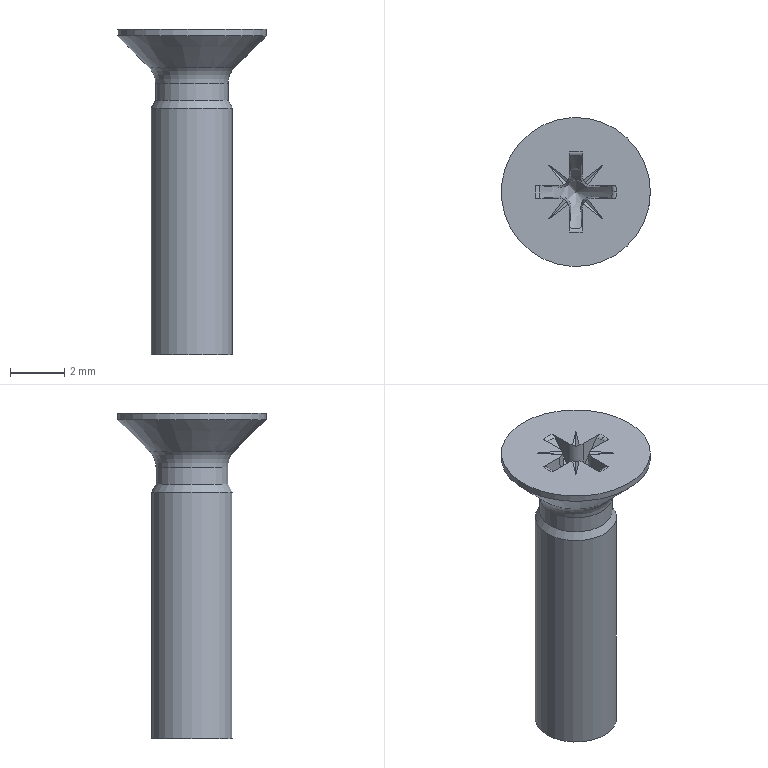Part | NX | features BREP 1, DATUM_CSYS 1 | 1 solid | 34 faces | box 5.5 x 5.5 x 12.001 mm | volume 94.702 mm3 | plane 18 | cylinder 7 | torus 6 | cone 3 | commonest cylinder face diameters 0.8 x4 2.675 x1 3 x1 5.5 x1
STEP:
#1=CARTESIAN_POINT('',(1.5,0.,-12.));
#2=VERTEX_POINT('',#1);
#3=CARTESIAN_POINT('',(0.,0.,-12.));
#4=DIRECTION('',(0.,0.,-1.));
#5=DIRECTION('',(1.,0.,0.));
#6=AXIS2_PLACEMENT_3D('',#3,#4,#5);
#7=CIRCLE('',#6,1.5);
#8=EDGE_CURVE('',#2,#2,#7,.T.);
#9=ORIENTED_EDGE('',*,*,#8,.T.);
#10=EDGE_LOOP('',(#9));
#11=FACE_BOUND('',#10,.T.);
#12=CARTESIAN_POINT('',(0.,0.,-12.));
#13=DIRECTION('',(0.,0.,-1.));
#14=DIRECTION('',(-1.,0.,0.));
#15=AXIS2_PLACEMENT_3D('',#12,#13,#14);
#16=PLANE('',#15);
#17=ADVANCED_FACE('',(#11),#16,.T.);
#18=CARTESIAN_POINT('',(1.5,0.,-2.9));
#19=VERTEX_POINT('',#18);
#20=CARTESIAN_POINT('',(1.5,0.,-12.));
#21=DIRECTION('',(0.,0.,1.));
#22=VECTOR('',#21,1000.);
#23=LINE('',#20,#22);
#24=EDGE_CURVE('',#2,#19,#23,.T.);
#25=ORIENTED_EDGE('',*,*,#24,.T.);
#26=CARTESIAN_POINT('',(0.,0.,-2.9));
#27=DIRECTION('',(0.,0.,-1.));
#28=DIRECTION('',(1.,0.,0.));
#29=AXIS2_PLACEMENT_3D('',#26,#27,#28);
#30=CIRCLE('',#29,1.5);
#31=EDGE_CURVE('',#19,#19,#30,.T.);
#32=ORIENTED_EDGE('',*,*,#31,.T.);
#33=ORIENTED_EDGE('',*,*,#24,.F.);
#34=ORIENTED_EDGE('',*,*,#8,.F.);
#35=EDGE_LOOP('',(#25,#32,#33,#34));
#36=FACE_BOUND('',#35,.T.);
#37=CARTESIAN_POINT('',(0.,0.,-12.));
#38=DIRECTION('',(0.,0.,1.));
#39=DIRECTION('',(-1.,0.,0.));
#40=AXIS2_PLACEMENT_3D('',#37,#38,#39);
#41=CYLINDRICAL_SURFACE('',#40,1.5);
#42=ADVANCED_FACE('',(#36),#41,.T.);
#43=CARTESIAN_POINT('',(1.338,0.,-2.619));
#44=VERTEX_POINT('',#43);
#45=CARTESIAN_POINT('',(1.5,0.,-2.9));
#46=DIRECTION('',(-0.5,0.,0.866));
#47=VECTOR('',#46,1000.);
#48=LINE('',#45,#47);
#49=EDGE_CURVE('',#19,#44,#48,.T.);
#50=ORIENTED_EDGE('',*,*,#49,.T.);
#51=CARTESIAN_POINT('',(0.,0.,-2.619));
#52=DIRECTION('',(0.,0.,-1.));
#53=DIRECTION('',(1.,0.,0.));
#54=AXIS2_PLACEMENT_3D('',#51,#52,#53);
#55=CIRCLE('',#54,1.338);
#56=EDGE_CURVE('',#44,#44,#55,.T.);
#57=ORIENTED_EDGE('',*,*,#56,.T.);
#58=ORIENTED_EDGE('',*,*,#49,.F.);
#59=ORIENTED_EDGE('',*,*,#31,.F.);
#60=EDGE_LOOP('',(#50,#57,#58,#59));
#61=FACE_BOUND('',#60,.T.);
#62=CARTESIAN_POINT('',(0.,0.,-2.619));
#63=DIRECTION('',(0.,0.,-1.));
#64=DIRECTION('',(-1.,0.,0.));
#65=AXIS2_PLACEMENT_3D('',#62,#63,#64);
#66=CONICAL_SURFACE('',#65,1.338,0.5236);
#67=ADVANCED_FACE('',(#61),#66,.T.);
#68=CARTESIAN_POINT('',(1.338,0.,-1.981));
#69=VERTEX_POINT('',#68);
#70=CARTESIAN_POINT('',(1.338,0.,-2.619));
#71=DIRECTION('',(0.,0.,1.));
#72=VECTOR('',#71,1000.);
#73=LINE('',#70,#72);
#74=EDGE_CURVE('',#44,#69,#73,.T.);
#75=ORIENTED_EDGE('',*,*,#74,.T.);
#76=CARTESIAN_POINT('',(0.,0.,-1.981));
#77=DIRECTION('',(0.,0.,-1.));
#78=DIRECTION('',(1.,0.,0.));
#79=AXIS2_PLACEMENT_3D('',#76,#77,#78);
#80=CIRCLE('',#79,1.338);
#81=EDGE_CURVE('',#69,#69,#80,.T.);
#82=ORIENTED_EDGE('',*,*,#81,.T.);
#83=ORIENTED_EDGE('',*,*,#74,.F.);
#84=ORIENTED_EDGE('',*,*,#56,.F.);
#85=EDGE_LOOP('',(#75,#82,#83,#84));
#86=FACE_BOUND('',#85,.T.);
#87=CARTESIAN_POINT('',(0.,0.,-2.619));
#88=DIRECTION('',(0.,0.,1.));
#89=DIRECTION('',(-1.,0.,0.));
#90=AXIS2_PLACEMENT_3D('',#87,#88,#89);
#91=CYLINDRICAL_SURFACE('',#90,1.338);
#92=ADVANCED_FACE('',(#86),#91,.T.);
#93=CARTESIAN_POINT('',(1.572,0.,-1.416));
#94=VERTEX_POINT('',#93);
#95=CARTESIAN_POINT('',(2.138,0.,-1.981));
#96=DIRECTION('',(0.,1.,0.));
#97=DIRECTION('',(-1.,0.,0.));
#98=AXIS2_PLACEMENT_3D('',#95,#96,#97);
#99=CIRCLE('',#98,0.8);
#100=EDGE_CURVE('',#69,#94,#99,.T.);
#101=ORIENTED_EDGE('',*,*,#100,.T.);
#102=CARTESIAN_POINT('',(0.,0.,-1.416));
#103=DIRECTION('',(0.,0.,-1.));
#104=DIRECTION('',(1.,0.,0.));
#105=AXIS2_PLACEMENT_3D('',#102,#103,#104);
#106=CIRCLE('',#105,1.572);
#107=EDGE_CURVE('',#94,#94,#106,.T.);
#108=ORIENTED_EDGE('',*,*,#107,.T.);
#109=ORIENTED_EDGE('',*,*,#100,.F.);
#110=ORIENTED_EDGE('',*,*,#81,.F.);
#111=EDGE_LOOP('',(#101,#108,#109,#110));
#112=FACE_BOUND('',#111,.T.);
#113=CARTESIAN_POINT('',(0.,0.,-1.981));
#114=DIRECTION('',(0.,0.,1.));
#115=DIRECTION('',(-1.,0.,0.));
#116=AXIS2_PLACEMENT_3D('',#113,#114,#115);
#117=TOROIDAL_SURFACE('',#116,2.138,0.8);
#118=ADVANCED_FACE('',(#112),#117,.F.);
#119=CARTESIAN_POINT('',(2.75,0.,-0.2376));
#120=VERTEX_POINT('',#119);
#121=CARTESIAN_POINT('',(1.572,0.,-1.416));
#122=DIRECTION('',(0.7071,0.,0.7071));
#123=VECTOR('',#122,1000.);
#124=LINE('',#121,#123);
#125=EDGE_CURVE('',#94,#120,#124,.T.);
#126=ORIENTED_EDGE('',*,*,#125,.T.);
#127=CARTESIAN_POINT('',(0.,0.,-0.2376));
#128=DIRECTION('',(0.,0.,-1.));
#129=DIRECTION('',(1.,0.,0.));
#130=AXIS2_PLACEMENT_3D('',#127,#128,#129);
#131=CIRCLE('',#130,2.75);
#132=EDGE_CURVE('',#120,#120,#131,.T.);
#133=ORIENTED_EDGE('',*,*,#132,.T.);
#134=ORIENTED_EDGE('',*,*,#125,.F.);
#135=ORIENTED_EDGE('',*,*,#107,.F.);
#136=EDGE_LOOP('',(#126,#133,#134,#135));
#137=FACE_BOUND('',#136,.T.);
#138=CARTESIAN_POINT('',(0.,0.,-1.416));
#139=DIRECTION('',(0.,0.,1.));
#140=DIRECTION('',(-1.,0.,0.));
#141=AXIS2_PLACEMENT_3D('',#138,#139,#140);
#142=CONICAL_SURFACE('',#141,1.572,0.7854);
#143=ADVANCED_FACE('',(#137),#142,.T.);
#144=CARTESIAN_POINT('',(2.75,0.,0.));
#145=VERTEX_POINT('',#144);
#146=CARTESIAN_POINT('',(2.75,0.,-0.2376));
#147=DIRECTION('',(0.,0.,1.));
#148=VECTOR('',#147,1000.);
#149=LINE('',#146,#148);
#150=EDGE_CURVE('',#120,#145,#149,.T.);
#151=ORIENTED_EDGE('',*,*,#150,.T.);
#152=CARTESIAN_POINT('',(0.,0.,0.));
#153=DIRECTION('',(0.,0.,-1.));
#154=DIRECTION('',(1.,0.,0.));
#155=AXIS2_PLACEMENT_3D('',#152,#153,#154);
#156=CIRCLE('',#155,2.75);
#157=EDGE_CURVE('',#145,#145,#156,.T.);
#158=ORIENTED_EDGE('',*,*,#157,.T.);
#159=ORIENTED_EDGE('',*,*,#150,.F.);
#160=ORIENTED_EDGE('',*,*,#132,.F.);
#161=EDGE_LOOP('',(#151,#158,#159,#160));
#162=FACE_BOUND('',#161,.T.);
#163=CARTESIAN_POINT('',(0.,0.,-0.2376));
#164=DIRECTION('',(0.,0.,1.));
#165=DIRECTION('',(-1.,0.,0.));
#166=AXIS2_PLACEMENT_3D('',#163,#164,#165);
#167=CYLINDRICAL_SURFACE('',#166,2.75);
#168=ADVANCED_FACE('',(#162),#167,.T.);
#169=ORIENTED_EDGE('',*,*,#157,.F.);
#170=EDGE_LOOP('',(#169));
#171=FACE_BOUND('',#170,.T.);
#172=CARTESIAN_POINT('',(-1.477,-0.2333,0.));
#173=VERTEX_POINT('',#172);
#174=CARTESIAN_POINT('',(-1.477,0.2333,0.));
#175=VERTEX_POINT('',#174);
#176=CARTESIAN_POINT('',(0.,0.,0.));
#177=DIRECTION('',(0.,0.,-1.));
#178=DIRECTION('',(-0.9878,-0.156,0.));
#179=AXIS2_PLACEMENT_3D('',#176,#177,#178);
#180=CIRCLE('',#179,1.495);
#181=EDGE_CURVE('',#173,#175,#180,.T.);
#182=ORIENTED_EDGE('',*,*,#181,.T.);
#183=CARTESIAN_POINT('',(-0.6328,0.2333,0.));
#184=VERTEX_POINT('',#183);
#185=CARTESIAN_POINT('',(-0.6328,0.2333,0.));
#186=DIRECTION('',(-1.,0.,0.));
#187=VECTOR('',#186,1000.);
#188=LINE('',#185,#187);
#189=EDGE_CURVE('',#184,#175,#188,.T.);
#190=ORIENTED_EDGE('',*,*,#189,.F.);
#191=CARTESIAN_POINT('',(-0.4469,0.2794,0.003653));
#192=VERTEX_POINT('',#191);
#193=CARTESIAN_POINT('',(-0.6339,0.6339,0.));
#194=DIRECTION('',(0.,0.,1.));
#195=DIRECTION('',(0.7071,-0.7071,0.));
#196=AXIS2_PLACEMENT_3D('',#193,#194,#195);
#197=ELLIPSE('',#196,0.4011,0.4);
#198=EDGE_CURVE('',#184,#192,#197,.T.);
#199=ORIENTED_EDGE('',*,*,#198,.T.);
#200=CARTESIAN_POINT('',(-0.9899,0.9899,0.));
#201=VERTEX_POINT('',#200);
#202=CARTESIAN_POINT('',(-0.9899,0.9899,0.));
#203=DIRECTION('',(0.6072,-0.7945,0.));
#204=VECTOR('',#203,1000.);
#205=LINE('',#202,#204);
#206=EDGE_CURVE('',#201,#192,#205,.T.);
#207=ORIENTED_EDGE('',*,*,#206,.F.);
#208=CARTESIAN_POINT('',(-0.2794,0.4469,0.003653));
#209=VERTEX_POINT('',#208);
#210=CARTESIAN_POINT('',(-0.2792,0.4467,0.));
#211=DIRECTION('',(-0.7945,0.6072,0.));
#212=VECTOR('',#211,1000.);
#213=LINE('',#210,#212);
#214=EDGE_CURVE('',#209,#201,#213,.T.);
#215=ORIENTED_EDGE('',*,*,#214,.F.);
#216=CARTESIAN_POINT('',(-0.2333,0.6328,0.));
#217=VERTEX_POINT('',#216);
#218=CARTESIAN_POINT('',(-0.6339,0.6339,0.));
#219=DIRECTION('',(0.,0.,1.));
#220=DIRECTION('',(0.7071,-0.7071,0.));
#221=AXIS2_PLACEMENT_3D('',#218,#219,#220);
#222=ELLIPSE('',#221,0.4011,0.4);
#223=EDGE_CURVE('',#209,#217,#222,.T.);
#224=ORIENTED_EDGE('',*,*,#223,.T.);
#225=CARTESIAN_POINT('',(-0.2333,1.477,0.));
#226=VERTEX_POINT('',#225);
#227=CARTESIAN_POINT('',(-0.2333,0.6328,0.));
#228=DIRECTION('',(0.,1.,0.));
#229=VECTOR('',#228,1000.);
#230=LINE('',#227,#229);
#231=EDGE_CURVE('',#217,#226,#230,.T.);
#232=ORIENTED_EDGE('',*,*,#231,.T.);
#233=CARTESIAN_POINT('',(0.2333,1.477,0.));
#234=VERTEX_POINT('',#233);
#235=CARTESIAN_POINT('',(0.,0.,0.));
#236=DIRECTION('',(0.,0.,-1.));
#237=DIRECTION('',(-0.156,0.9878,0.));
#238=AXIS2_PLACEMENT_3D('',#235,#236,#237);
#239=CIRCLE('',#238,1.495);
#240=EDGE_CURVE('',#226,#234,#239,.T.);
#241=ORIENTED_EDGE('',*,*,#240,.T.);
#242=CARTESIAN_POINT('',(0.2333,0.6328,0.));
#243=VERTEX_POINT('',#242);
#244=CARTESIAN_POINT('',(0.2333,0.6328,0.));
#245=DIRECTION('',(0.,1.,0.));
#246=VECTOR('',#245,1000.);
#247=LINE('',#244,#246);
#248=EDGE_CURVE('',#243,#234,#247,.T.);
#249=ORIENTED_EDGE('',*,*,#248,.F.);
#250=CARTESIAN_POINT('',(0.2794,0.4469,0.003653));
#251=VERTEX_POINT('',#250);
#252=CARTESIAN_POINT('',(0.6339,0.6339,0.));
#253=DIRECTION('',(0.,0.,1.));
#254=DIRECTION('',(-0.7071,-0.7071,0.));
#255=AXIS2_PLACEMENT_3D('',#252,#253,#254);
#256=ELLIPSE('',#255,0.4011,0.4);
#257=EDGE_CURVE('',#243,#251,#256,.T.);
#258=ORIENTED_EDGE('',*,*,#257,.T.);
#259=CARTESIAN_POINT('',(0.9899,0.9899,0.));
#260=VERTEX_POINT('',#259);
#261=CARTESIAN_POINT('',(0.9899,0.9899,0.));
#262=DIRECTION('',(-0.7945,-0.6072,0.));
#263=VECTOR('',#262,1000.);
#264=LINE('',#261,#263);
#265=EDGE_CURVE('',#260,#251,#264,.T.);
#266=ORIENTED_EDGE('',*,*,#265,.F.);
#267=CARTESIAN_POINT('',(0.4469,0.2794,0.003653));
#268=VERTEX_POINT('',#267);
#269=CARTESIAN_POINT('',(0.4467,0.2792,0.));
#270=DIRECTION('',(0.6072,0.7945,0.));
#271=VECTOR('',#270,1000.);
#272=LINE('',#269,#271);
#273=EDGE_CURVE('',#268,#260,#272,.T.);
#274=ORIENTED_EDGE('',*,*,#273,.F.);
#275=CARTESIAN_POINT('',(0.6328,0.2333,0.));
#276=VERTEX_POINT('',#275);
#277=CARTESIAN_POINT('',(0.6339,0.6339,0.));
#278=DIRECTION('',(0.,0.,1.));
#279=DIRECTION('',(-0.7071,-0.7071,0.));
#280=AXIS2_PLACEMENT_3D('',#277,#278,#279);
#281=ELLIPSE('',#280,0.4011,0.4);
#282=EDGE_CURVE('',#268,#276,#281,.T.);
#283=ORIENTED_EDGE('',*,*,#282,.T.);
#284=CARTESIAN_POINT('',(1.477,0.2333,0.));
#285=VERTEX_POINT('',#284);
#286=CARTESIAN_POINT('',(0.6328,0.2333,0.));
#287=DIRECTION('',(1.,0.,0.));
#288=VECTOR('',#287,1000.);
#289=LINE('',#286,#288);
#290=EDGE_CURVE('',#276,#285,#289,.T.);
#291=ORIENTED_EDGE('',*,*,#290,.T.);
#292=CARTESIAN_POINT('',(1.495,0.,0.));
#293=VERTEX_POINT('',#292);
#294=CARTESIAN_POINT('',(0.,0.,0.));
#295=DIRECTION('',(0.,0.,-1.));
#296=DIRECTION('',(0.9878,0.156,0.));
#297=AXIS2_PLACEMENT_3D('',#294,#295,#296);
#298=CIRCLE('',#297,1.495);
#299=EDGE_CURVE('',#285,#293,#298,.T.);
#300=ORIENTED_EDGE('',*,*,#299,.T.);
#301=CARTESIAN_POINT('',(1.477,-0.2333,0.));
#302=VERTEX_POINT('',#301);
#303=CARTESIAN_POINT('',(0.,0.,0.));
#304=DIRECTION('',(0.,0.,-1.));
#305=DIRECTION('',(1.,0.,0.));
#306=AXIS2_PLACEMENT_3D('',#303,#304,#305);
#307=CIRCLE('',#306,1.495);
#308=EDGE_CURVE('',#293,#302,#307,.T.);
#309=ORIENTED_EDGE('',*,*,#308,.T.);
#310=CARTESIAN_POINT('',(0.6328,-0.2333,0.));
#311=VERTEX_POINT('',#310);
#312=CARTESIAN_POINT('',(0.6328,-0.2333,0.));
#313=DIRECTION('',(1.,0.,0.));
#314=VECTOR('',#313,1000.);
#315=LINE('',#312,#314);
#316=EDGE_CURVE('',#311,#302,#315,.T.);
#317=ORIENTED_EDGE('',*,*,#316,.F.);
#318=CARTESIAN_POINT('',(0.4469,-0.2794,0.003653));
#319=VERTEX_POINT('',#318);
#320=CARTESIAN_POINT('',(0.6339,-0.6339,0.));
#321=DIRECTION('',(0.,0.,1.));
#322=DIRECTION('',(-0.7071,0.7071,0.));
#323=AXIS2_PLACEMENT_3D('',#320,#321,#322);
#324=ELLIPSE('',#323,0.4011,0.4);
#325=EDGE_CURVE('',#311,#319,#324,.T.);
#326=ORIENTED_EDGE('',*,*,#325,.T.);
#327=CARTESIAN_POINT('',(0.9899,-0.9899,0.));
#328=VERTEX_POINT('',#327);
#329=CARTESIAN_POINT('',(0.9899,-0.9899,0.));
#330=DIRECTION('',(-0.6072,0.7945,0.));
#331=VECTOR('',#330,1000.);
#332=LINE('',#329,#331);
#333=EDGE_CURVE('',#328,#319,#332,.T.);
#334=ORIENTED_EDGE('',*,*,#333,.F.);
#335=CARTESIAN_POINT('',(0.2794,-0.4469,0.003653));
#336=VERTEX_POINT('',#335);
#337=CARTESIAN_POINT('',(0.2792,-0.4467,0.));
#338=DIRECTION('',(0.7945,-0.6072,0.));
#339=VECTOR('',#338,1000.);
#340=LINE('',#337,#339);
#341=EDGE_CURVE('',#336,#328,#340,.T.);
#342=ORIENTED_EDGE('',*,*,#341,.F.);
#343=CARTESIAN_POINT('',(0.2333,-0.6328,0.));
#344=VERTEX_POINT('',#343);
#345=CARTESIAN_POINT('',(0.6339,-0.6339,0.));
#346=DIRECTION('',(0.,0.,1.));
#347=DIRECTION('',(-0.7071,0.7071,0.));
#348=AXIS2_PLACEMENT_3D('',#345,#346,#347);
#349=ELLIPSE('',#348,0.4011,0.4);
#350=EDGE_CURVE('',#336,#344,#349,.T.);
#351=ORIENTED_EDGE('',*,*,#350,.T.);
#352=CARTESIAN_POINT('',(0.2333,-1.477,0.));
#353=VERTEX_POINT('',#352);
#354=CARTESIAN_POINT('',(0.2333,-0.6328,0.));
#355=DIRECTION('',(0.,-1.,0.));
#356=VECTOR('',#355,1000.);
#357=LINE('',#354,#356);
#358=EDGE_CURVE('',#344,#353,#357,.T.);
#359=ORIENTED_EDGE('',*,*,#358,.T.);
#360=CARTESIAN_POINT('',(-0.2333,-1.477,0.));
#361=VERTEX_POINT('',#360);
#362=CARTESIAN_POINT('',(0.,0.,0.));
#363=DIRECTION('',(0.,0.,-1.));
#364=DIRECTION('',(0.156,-0.9878,0.));
#365=AXIS2_PLACEMENT_3D('',#362,#363,#364);
#366=CIRCLE('',#365,1.495);
#367=EDGE_CURVE('',#353,#361,#366,.T.);
#368=ORIENTED_EDGE('',*,*,#367,.T.);
#369=CARTESIAN_POINT('',(-0.2333,-0.6328,0.));
#370=VERTEX_POINT('',#369);
#371=CARTESIAN_POINT('',(-0.2333,-0.6328,0.));
#372=DIRECTION('',(0.,-1.,0.));
#373=VECTOR('',#372,1000.);
#374=LINE('',#371,#373);
#375=EDGE_CURVE('',#370,#361,#374,.T.);
#376=ORIENTED_EDGE('',*,*,#375,.F.);
#377=CARTESIAN_POINT('',(-0.2794,-0.4469,0.003653));
#378=VERTEX_POINT('',#377);
#379=CARTESIAN_POINT('',(-0.6339,-0.6339,0.));
#380=DIRECTION('',(0.,0.,1.));
#381=DIRECTION('',(0.7071,0.7071,0.));
#382=AXIS2_PLACEMENT_3D('',#379,#380,#381);
#383=ELLIPSE('',#382,0.4011,0.4);
#384=EDGE_CURVE('',#370,#378,#383,.T.);
#385=ORIENTED_EDGE('',*,*,#384,.T.);
#386=CARTESIAN_POINT('',(-0.9899,-0.9899,0.));
#387=VERTEX_POINT('',#386);
#388=CARTESIAN_POINT('',(-0.9899,-0.9899,0.));
#389=DIRECTION('',(0.7945,0.6072,0.));
#390=VECTOR('',#389,1000.);
#391=LINE('',#388,#390);
#392=EDGE_CURVE('',#387,#378,#391,.T.);
#393=ORIENTED_EDGE('',*,*,#392,.F.);
#394=CARTESIAN_POINT('',(-0.4469,-0.2794,0.003653));
#395=VERTEX_POINT('',#394);
#396=CARTESIAN_POINT('',(-0.4467,-0.2792,0.));
#397=DIRECTION('',(-0.6072,-0.7945,0.));
#398=VECTOR('',#397,1000.);
#399=LINE('',#396,#398);
#400=EDGE_CURVE('',#395,#387,#399,.T.);
#401=ORIENTED_EDGE('',*,*,#400,.F.);
#402=CARTESIAN_POINT('',(-0.6328,-0.2333,0.));
#403=VERTEX_POINT('',#402);
#404=CARTESIAN_POINT('',(-0.6339,-0.6339,0.));
#405=DIRECTION('',(0.,0.,1.));
#406=DIRECTION('',(0.7071,0.7071,0.));
#407=AXIS2_PLACEMENT_3D('',#404,#405,#406);
#408=ELLIPSE('',#407,0.4011,0.4);
#409=EDGE_CURVE('',#395,#403,#408,.T.);
#410=ORIENTED_EDGE('',*,*,#409,.T.);
#411=CARTESIAN_POINT('',(-0.6328,-0.2333,0.));
#412=DIRECTION('',(-1.,0.,0.));
#413=VECTOR('',#412,1000.);
#414=LINE('',#411,#413);
#415=EDGE_CURVE('',#403,#173,#414,.T.);
#416=ORIENTED_EDGE('',*,*,#415,.T.);
#417=EDGE_LOOP('',(#182,#190,#199,#207,#215,#224,#232,#241,#249,#258,#266,#274,#283,#291,#300,#309,#317,#326,#334,#342,#351,#359,#368,#376,#385,#393,#401,#410,#416));
#418=FACE_BOUND('',#417,.T.);
#419=CARTESIAN_POINT('',(0.,0.,0.));
#420=DIRECTION('',(0.,0.,1.));
#421=DIRECTION('',(-1.,0.,0.));
#422=AXIS2_PLACEMENT_3D('',#419,#420,#421);
#423=PLANE('',#422);
#424=ADVANCED_FACE('',(#171,#418),#423,.T.);
#425=CARTESIAN_POINT('',(1.34,0.,-0.07419));
#426=VERTEX_POINT('',#425);
#427=CARTESIAN_POINT('',(0.,0.,-1.73));
#428=VERTEX_POINT('',#427);
#429=CARTESIAN_POINT('',(1.34,0.,-0.07419));
#430=DIRECTION('',(-0.6291,0.,-0.7773));
#431=VECTOR('',#430,1000.);
#432=LINE('',#429,#431);
#433=EDGE_CURVE('',#426,#428,#432,.T.);
#434=ORIENTED_EDGE('',*,*,#433,.F.);
#435=CARTESIAN_POINT('',(1.32,0.2294,-0.07419));
#436=VERTEX_POINT('',#435);
#437=CARTESIAN_POINT('',(0.,0.,-0.07419));
#438=DIRECTION('',(0.,0.,-1.));
#439=DIRECTION('',(0.9852,0.1712,0.));
#440=AXIS2_PLACEMENT_3D('',#437,#438,#439);
#441=CIRCLE('',#440,1.34);
#442=EDGE_CURVE('',#436,#426,#441,.T.);
#443=ORIENTED_EDGE('',*,*,#442,.F.);
#444=CARTESIAN_POINT('',(0.5816,0.1821,-0.9769));
#445=VERTEX_POINT('',#444);
#446=CARTESIAN_POINT('',(1.32,0.2294,-0.07419));
#447=CARTESIAN_POINT('',(0.8112,0.1966,-0.7008));
#448=CARTESIAN_POINT('',(0.5816,0.1821,-0.9769));
#449=(BOUNDED_CURVE()B_SPLINE_CURVE(2,(#446,#447,#448),.UNSPECIFIED.,.F.,.F.)B_SPLINE_CURVE_WITH_KNOTS((3,3),(0.,1.),.PIECEWISE_BEZIER_KNOTS.)CURVE()GEOMETRIC_REPRESENTATION_ITEM()RATIONAL_B_SPLINE_CURVE((1.041,1.587,2.063))REPRESENTATION_ITEM(''));
#450=EDGE_CURVE('',#436,#445,#449,.T.);
#451=ORIENTED_EDGE('',*,*,#450,.T.);
#452=CARTESIAN_POINT('',(0.1821,0.5816,-0.9769));
#453=VERTEX_POINT('',#452);
#454=CARTESIAN_POINT('',(0.1821,0.5816,-0.9769));
#455=CARTESIAN_POINT('',(0.1765,0.4916,-1.085));
#456=CARTESIAN_POINT('',(0.2377,0.2374,-1.376));
#457=CARTESIAN_POINT('',(0.4916,0.1765,-1.085));
#458=CARTESIAN_POINT('',(0.5816,0.1821,-0.9769));
#459=B_SPLINE_CURVE_WITH_KNOTS('',3,(#454,#455,#456,#457,#458),.UNSPECIFIED.,.F.,.F.,(4,1,4),(0.,0.0004195,0.000839),.UNSPECIFIED.);
#460=EDGE_CURVE('',#453,#445,#459,.T.);
#461=ORIENTED_EDGE('',*,*,#460,.F.);
#462=CARTESIAN_POINT('',(0.2294,1.32,-0.07419));
#463=VERTEX_POINT('',#462);
#464=CARTESIAN_POINT('',(0.1821,0.5816,-0.9769));
#465=CARTESIAN_POINT('',(0.1966,0.8112,-0.7008));
#466=CARTESIAN_POINT('',(0.2294,1.32,-0.07419));
#467=(BOUNDED_CURVE()B_SPLINE_CURVE(2,(#464,#465,#466),.UNSPECIFIED.,.F.,.F.)B_SPLINE_CURVE_WITH_KNOTS((3,3),(0.,1.),.PIECEWISE_BEZIER_KNOTS.)CURVE()GEOMETRIC_REPRESENTATION_ITEM()RATIONAL_B_SPLINE_CURVE((2.063,1.587,1.041))REPRESENTATION_ITEM(''));
#468=EDGE_CURVE('',#453,#463,#467,.T.);
#469=ORIENTED_EDGE('',*,*,#468,.T.);
#470=CARTESIAN_POINT('',(-0.2294,1.32,-0.07419));
#471=VERTEX_POINT('',#470);
#472=CARTESIAN_POINT('',(0.,0.,-0.07419));
#473=DIRECTION('',(0.,0.,-1.));
#474=DIRECTION('',(-0.1712,0.9852,0.));
#475=AXIS2_PLACEMENT_3D('',#472,#473,#474);
#476=CIRCLE('',#475,1.34);
#477=EDGE_CURVE('',#471,#463,#476,.T.);
#478=ORIENTED_EDGE('',*,*,#477,.F.);
#479=CARTESIAN_POINT('',(-0.1821,0.5816,-0.9769));
#480=VERTEX_POINT('',#479);
#481=CARTESIAN_POINT('',(-0.2294,1.32,-0.07419));
#482=CARTESIAN_POINT('',(-0.1966,0.8112,-0.7008));
#483=CARTESIAN_POINT('',(-0.1821,0.5816,-0.9769));
#484=(BOUNDED_CURVE()B_SPLINE_CURVE(2,(#481,#482,#483),.UNSPECIFIED.,.F.,.F.)B_SPLINE_CURVE_WITH_KNOTS((3,3),(0.,1.),.PIECEWISE_BEZIER_KNOTS.)CURVE()GEOMETRIC_REPRESENTATION_ITEM()RATIONAL_B_SPLINE_CURVE((1.041,1.587,2.063))REPRESENTATION_ITEM(''));
#485=EDGE_CURVE('',#471,#480,#484,.T.);
#486=ORIENTED_EDGE('',*,*,#485,.T.);
#487=CARTESIAN_POINT('',(-0.5816,0.1821,-0.9769));
#488=VERTEX_POINT('',#487);
#489=CARTESIAN_POINT('',(-0.5816,0.1821,-0.9769));
#490=CARTESIAN_POINT('',(-0.4916,0.1765,-1.085));
#491=CARTESIAN_POINT('',(-0.2374,0.2377,-1.376));
#492=CARTESIAN_POINT('',(-0.1765,0.4916,-1.085));
#493=CARTESIAN_POINT('',(-0.1821,0.5816,-0.9769));
#494=B_SPLINE_CURVE_WITH_KNOTS('',3,(#489,#490,#491,#492,#493),.UNSPECIFIED.,.F.,.F.,(4,1,4),(0.,0.0004195,0.000839),.UNSPECIFIED.);
#495=EDGE_CURVE('',#488,#480,#494,.T.);
#496=ORIENTED_EDGE('',*,*,#495,.F.);
#497=CARTESIAN_POINT('',(-1.32,0.2294,-0.07419));
#498=VERTEX_POINT('',#497);
#499=CARTESIAN_POINT('',(-0.5816,0.1821,-0.9769));
#500=CARTESIAN_POINT('',(-0.8112,0.1966,-0.7008));
#501=CARTESIAN_POINT('',(-1.32,0.2294,-0.07419));
#502=(BOUNDED_CURVE()B_SPLINE_CURVE(2,(#499,#500,#501),.UNSPECIFIED.,.F.,.F.)B_SPLINE_CURVE_WITH_KNOTS((3,3),(0.,1.),.PIECEWISE_BEZIER_KNOTS.)CURVE()GEOMETRIC_REPRESENTATION_ITEM()RATIONAL_B_SPLINE_CURVE((2.063,1.587,1.041))REPRESENTATION_ITEM(''));
#503=EDGE_CURVE('',#488,#498,#502,.T.);
#504=ORIENTED_EDGE('',*,*,#503,.T.);
#505=CARTESIAN_POINT('',(-1.32,-0.2294,-0.07419));
#506=VERTEX_POINT('',#505);
#507=CARTESIAN_POINT('',(0.,0.,-0.07419));
#508=DIRECTION('',(0.,0.,-1.));
#509=DIRECTION('',(-0.9852,-0.1712,0.));
#510=AXIS2_PLACEMENT_3D('',#507,#508,#509);
#511=CIRCLE('',#510,1.34);
#512=EDGE_CURVE('',#506,#498,#511,.T.);
#513=ORIENTED_EDGE('',*,*,#512,.F.);
#514=CARTESIAN_POINT('',(-0.5816,-0.1821,-0.9769));
#515=VERTEX_POINT('',#514);
#516=CARTESIAN_POINT('',(-1.32,-0.2294,-0.07419));
#517=CARTESIAN_POINT('',(-0.8112,-0.1966,-0.7008));
#518=CARTESIAN_POINT('',(-0.5816,-0.1821,-0.9769));
#519=(BOUNDED_CURVE()B_SPLINE_CURVE(2,(#516,#517,#518),.UNSPECIFIED.,.F.,.F.)B_SPLINE_CURVE_WITH_KNOTS((3,3),(0.,1.),.PIECEWISE_BEZIER_KNOTS.)CURVE()GEOMETRIC_REPRESENTATION_ITEM()RATIONAL_B_SPLINE_CURVE((1.041,1.587,2.063))REPRESENTATION_ITEM(''));
#520=EDGE_CURVE('',#506,#515,#519,.T.);
#521=ORIENTED_EDGE('',*,*,#520,.T.);
#522=CARTESIAN_POINT('',(-0.1821,-0.5816,-0.9769));
#523=VERTEX_POINT('',#522);
#524=CARTESIAN_POINT('',(-0.1821,-0.5816,-0.9769));
#525=CARTESIAN_POINT('',(-0.1765,-0.4916,-1.085));
#526=CARTESIAN_POINT('',(-0.2377,-0.2374,-1.376));
#527=CARTESIAN_POINT('',(-0.4916,-0.1765,-1.085));
#528=CARTESIAN_POINT('',(-0.5816,-0.1821,-0.9769));
#529=B_SPLINE_CURVE_WITH_KNOTS('',3,(#524,#525,#526,#527,#528),.UNSPECIFIED.,.F.,.F.,(4,1,4),(0.,0.0004195,0.000839),.UNSPECIFIED.);
#530=EDGE_CURVE('',#523,#515,#529,.T.);
#531=ORIENTED_EDGE('',*,*,#530,.F.);
#532=CARTESIAN_POINT('',(-0.2294,-1.32,-0.07419));
#533=VERTEX_POINT('',#532);
#534=CARTESIAN_POINT('',(-0.1821,-0.5816,-0.9769));
#535=CARTESIAN_POINT('',(-0.1966,-0.8112,-0.7008));
#536=CARTESIAN_POINT('',(-0.2294,-1.32,-0.07419));
#537=(BOUNDED_CURVE()B_SPLINE_CURVE(2,(#534,#535,#536),.UNSPECIFIED.,.F.,.F.)B_SPLINE_CURVE_WITH_KNOTS((3,3),(0.,1.),.PIECEWISE_BEZIER_KNOTS.)CURVE()GEOMETRIC_REPRESENTATION_ITEM()RATIONAL_B_SPLINE_CURVE((2.063,1.587,1.041))REPRESENTATION_ITEM(''));
#538=EDGE_CURVE('',#523,#533,#537,.T.);
#539=ORIENTED_EDGE('',*,*,#538,.T.);
#540=CARTESIAN_POINT('',(0.2294,-1.32,-0.07419));
#541=VERTEX_POINT('',#540);
#542=CARTESIAN_POINT('',(0.,0.,-0.07419));
#543=DIRECTION('',(0.,0.,-1.));
#544=DIRECTION('',(0.1712,-0.9852,0.));
#545=AXIS2_PLACEMENT_3D('',#542,#543,#544);
#546=CIRCLE('',#545,1.34);
#547=EDGE_CURVE('',#541,#533,#546,.T.);
#548=ORIENTED_EDGE('',*,*,#547,.F.);
#549=CARTESIAN_POINT('',(0.1821,-0.5816,-0.9769));
#550=VERTEX_POINT('',#549);
#551=CARTESIAN_POINT('',(0.2294,-1.32,-0.07419));
#552=CARTESIAN_POINT('',(0.1966,-0.8112,-0.7008));
#553=CARTESIAN_POINT('',(0.1821,-0.5816,-0.9769));
#554=(BOUNDED_CURVE()B_SPLINE_CURVE(2,(#551,#552,#553),.UNSPECIFIED.,.F.,.F.)B_SPLINE_CURVE_WITH_KNOTS((3,3),(0.,1.),.PIECEWISE_BEZIER_KNOTS.)CURVE()GEOMETRIC_REPRESENTATION_ITEM()RATIONAL_B_SPLINE_CURVE((1.041,1.587,2.063))REPRESENTATION_ITEM(''));
#555=EDGE_CURVE('',#541,#550,#554,.T.);
#556=ORIENTED_EDGE('',*,*,#555,.T.);
#557=CARTESIAN_POINT('',(0.5816,-0.1821,-0.9769));
#558=VERTEX_POINT('',#557);
#559=CARTESIAN_POINT('',(0.5816,-0.1821,-0.9769));
#560=CARTESIAN_POINT('',(0.4916,-0.1765,-1.085));
#561=CARTESIAN_POINT('',(0.2374,-0.2377,-1.376));
#562=CARTESIAN_POINT('',(0.1765,-0.4916,-1.085));
#563=CARTESIAN_POINT('',(0.1821,-0.5816,-0.9769));
#564=B_SPLINE_CURVE_WITH_KNOTS('',3,(#559,#560,#561,#562,#563),.UNSPECIFIED.,.F.,.F.,(4,1,4),(0.,0.0004195,0.000839),.UNSPECIFIED.);
#565=EDGE_CURVE('',#558,#550,#564,.T.);
#566=ORIENTED_EDGE('',*,*,#565,.F.);
#567=CARTESIAN_POINT('',(1.32,-0.2294,-0.07419));
#568=VERTEX_POINT('',#567);
#569=CARTESIAN_POINT('',(0.5816,-0.1821,-0.9769));
#570=CARTESIAN_POINT('',(0.8112,-0.1966,-0.7008));
#571=CARTESIAN_POINT('',(1.32,-0.2294,-0.07419));
#572=(BOUNDED_CURVE()B_SPLINE_CURVE(2,(#569,#570,#571),.UNSPECIFIED.,.F.,.F.)B_SPLINE_CURVE_WITH_KNOTS((3,3),(0.,1.),.PIECEWISE_BEZIER_KNOTS.)CURVE()GEOMETRIC_REPRESENTATION_ITEM()RATIONAL_B_SPLINE_CURVE((2.063,1.587,1.041))REPRESENTATION_ITEM(''));
#573=EDGE_CURVE('',#558,#568,#572,.T.);
#574=ORIENTED_EDGE('',*,*,#573,.T.);
#575=CARTESIAN_POINT('',(0.,0.,-0.07419));
#576=DIRECTION('',(0.,0.,-1.));
#577=DIRECTION('',(1.,0.,0.));
#578=AXIS2_PLACEMENT_3D('',#575,#576,#577);
#579=CIRCLE('',#578,1.34);
#580=EDGE_CURVE('',#426,#568,#579,.T.);
#581=ORIENTED_EDGE('',*,*,#580,.F.);
#582=ORIENTED_EDGE('',*,*,#433,.T.);
#583=EDGE_LOOP('',(#434,#443,#451,#461,#469,#478,#486,#496,#504,#513,#521,#531,#539,#548,#556,#566,#574,#581,#582));
#584=FACE_BOUND('',#583,.T.);
#585=CARTESIAN_POINT('',(0.,0.,-1.73));
#586=DIRECTION('',(0.,0.,1.));
#587=DIRECTION('',(-1.,0.,0.));
#588=AXIS2_PLACEMENT_3D('',#585,#586,#587);
#589=CONICAL_SURFACE('',#588,0.,0.6804);
#590=ADVANCED_FACE('',(#584),#589,.F.);
#591=CARTESIAN_POINT('',(-1.32,-0.2294,-0.07419));
#592=CARTESIAN_POINT('',(-1.358,-0.2319,-0.02705));
#593=CARTESIAN_POINT('',(-1.416,-0.2333,0.));
#594=CARTESIAN_POINT('',(-1.477,-0.2333,0.));
#595=B_SPLINE_CURVE_WITH_KNOTS('',3,(#591,#592,#593,#594),.UNSPECIFIED.,.F.,.F.,(4,4),(0.,1.),.PIECEWISE_BEZIER_KNOTS.);
#596=EDGE_CURVE('',#506,#173,#595,.T.);
#597=ORIENTED_EDGE('',*,*,#596,.T.);
#598=ORIENTED_EDGE('',*,*,#415,.F.);
#599=CARTESIAN_POINT('',(-0.6328,-0.2333,0.));
#600=DIRECTION('',(0.05226,0.05226,-0.9973));
#601=VECTOR('',#600,1000.);
#602=LINE('',#599,#601);
#603=EDGE_CURVE('',#403,#515,#602,.T.);
#604=ORIENTED_EDGE('',*,*,#603,.T.);
#605=ORIENTED_EDGE('',*,*,#520,.F.);
#606=EDGE_LOOP('',(#597,#598,#604,#605));
#607=FACE_BOUND('',#606,.T.);
#608=CARTESIAN_POINT('',(-0.8171,-0.1952,-0.7278));
#609=DIRECTION('',(0.,-0.9986,-0.05234));
#610=DIRECTION('',(1.,0.,0.));
#611=AXIS2_PLACEMENT_3D('',#608,#609,#610);
#612=PLANE('',#611);
#613=ADVANCED_FACE('',(#607),#612,.F.);
#614=ORIENTED_EDGE('',*,*,#538,.F.);
#615=CARTESIAN_POINT('',(-0.2333,-0.6328,0.));
#616=DIRECTION('',(0.05226,0.05226,-0.9973));
#617=VECTOR('',#616,1000.);
#618=LINE('',#615,#617);
#619=EDGE_CURVE('',#370,#523,#618,.T.);
#620=ORIENTED_EDGE('',*,*,#619,.F.);
#621=ORIENTED_EDGE('',*,*,#375,.T.);
#622=CARTESIAN_POINT('',(-0.2294,-1.32,-0.07419));
#623=CARTESIAN_POINT('',(-0.2319,-1.358,-0.02705));
#624=CARTESIAN_POINT('',(-0.2333,-1.416,0.));
#625=CARTESIAN_POINT('',(-0.2333,-1.477,0.));
#626=B_SPLINE_CURVE_WITH_KNOTS('',3,(#622,#623,#624,#625),.UNSPECIFIED.,.F.,.F.,(4,4),(0.,1.),.PIECEWISE_BEZIER_KNOTS.);
#627=EDGE_CURVE('',#533,#361,#626,.T.);
#628=ORIENTED_EDGE('',*,*,#627,.F.);
#629=EDGE_LOOP('',(#614,#620,#621,#628));
#630=FACE_BOUND('',#629,.T.);
#631=CARTESIAN_POINT('',(-0.1952,-0.8171,-0.7278));
#632=DIRECTION('',(-0.9986,0.,-0.05234));
#633=DIRECTION('',(0.,-1.,0.));
#634=AXIS2_PLACEMENT_3D('',#631,#632,#633);
#635=PLANE('',#634);
#636=ADVANCED_FACE('',(#630),#635,.F.);
#637=CARTESIAN_POINT('',(0.2294,-1.32,-0.07419));
#638=CARTESIAN_POINT('',(0.2319,-1.358,-0.02705));
#639=CARTESIAN_POINT('',(0.2333,-1.416,0.));
#640=CARTESIAN_POINT('',(0.2333,-1.477,0.));
#641=B_SPLINE_CURVE_WITH_KNOTS('',3,(#637,#638,#639,#640),.UNSPECIFIED.,.F.,.F.,(4,4),(0.,1.),.PIECEWISE_BEZIER_KNOTS.);
#642=EDGE_CURVE('',#541,#353,#641,.T.);
#643=ORIENTED_EDGE('',*,*,#642,.T.);
#644=ORIENTED_EDGE('',*,*,#358,.F.);
#645=CARTESIAN_POINT('',(0.2333,-0.6328,0.));
#646=DIRECTION('',(-0.05226,0.05226,-0.9973));
#647=VECTOR('',#646,1000.);
#648=LINE('',#645,#647);
#649=EDGE_CURVE('',#344,#550,#648,.T.);
#650=ORIENTED_EDGE('',*,*,#649,.T.);
#651=ORIENTED_EDGE('',*,*,#555,.F.);
#652=EDGE_LOOP('',(#643,#644,#650,#651));
#653=FACE_BOUND('',#652,.T.);
#654=CARTESIAN_POINT('',(0.1952,-0.8171,-0.7278));
#655=DIRECTION('',(0.9986,0.,-0.05234));
#656=DIRECTION('',(0.,1.,0.));
#657=AXIS2_PLACEMENT_3D('',#654,#655,#656);
#658=PLANE('',#657);
#659=ADVANCED_FACE('',(#653),#658,.F.);
#660=ORIENTED_EDGE('',*,*,#573,.F.);
#661=CARTESIAN_POINT('',(0.6328,-0.2333,0.));
#662=DIRECTION('',(-0.05226,0.05226,-0.9973));
#663=VECTOR('',#662,1000.);
#664=LINE('',#661,#663);
#665=EDGE_CURVE('',#311,#558,#664,.T.);
#666=ORIENTED_EDGE('',*,*,#665,.F.);
#667=ORIENTED_EDGE('',*,*,#316,.T.);
#668=CARTESIAN_POINT('',(1.32,-0.2294,-0.07419));
#669=CARTESIAN_POINT('',(1.358,-0.2319,-0.02705));
#670=CARTESIAN_POINT('',(1.416,-0.2333,0.));
#671=CARTESIAN_POINT('',(1.477,-0.2333,0.));
#672=B_SPLINE_CURVE_WITH_KNOTS('',3,(#668,#669,#670,#671),.UNSPECIFIED.,.F.,.F.,(4,4),(0.,1.),.PIECEWISE_BEZIER_KNOTS.);
#673=EDGE_CURVE('',#568,#302,#672,.T.);
#674=ORIENTED_EDGE('',*,*,#673,.F.);
#675=EDGE_LOOP('',(#660,#666,#667,#674));
#676=FACE_BOUND('',#675,.T.);
#677=CARTESIAN_POINT('',(0.8171,-0.1952,-0.7278));
#678=DIRECTION('',(0.,-0.9986,-0.05234));
#679=DIRECTION('',(1.,0.,0.));
#680=AXIS2_PLACEMENT_3D('',#677,#678,#679);
#681=PLANE('',#680);
#682=ADVANCED_FACE('',(#676),#681,.F.);
#683=CARTESIAN_POINT('',(1.32,0.2294,-0.07419));
#684=CARTESIAN_POINT('',(1.358,0.2319,-0.02705));
#685=CARTESIAN_POINT('',(1.416,0.2333,0.));
#686=CARTESIAN_POINT('',(1.477,0.2333,0.));
#687=B_SPLINE_CURVE_WITH_KNOTS('',3,(#683,#684,#685,#686),.UNSPECIFIED.,.F.,.F.,(4,4),(0.,1.),.PIECEWISE_BEZIER_KNOTS.);
#688=EDGE_CURVE('',#436,#285,#687,.T.);
#689=ORIENTED_EDGE('',*,*,#688,.T.);
#690=ORIENTED_EDGE('',*,*,#290,.F.);
#691=CARTESIAN_POINT('',(0.6328,0.2333,0.));
#692=DIRECTION('',(-0.05226,-0.05226,-0.9973));
#693=VECTOR('',#692,1000.);
#694=LINE('',#691,#693);
#695=EDGE_CURVE('',#276,#445,#694,.T.);
#696=ORIENTED_EDGE('',*,*,#695,.T.);
#697=ORIENTED_EDGE('',*,*,#450,.F.);
#698=EDGE_LOOP('',(#689,#690,#696,#697));
#699=FACE_BOUND('',#698,.T.);
#700=CARTESIAN_POINT('',(0.8171,0.1952,-0.7278));
#701=DIRECTION('',(0.,0.9986,-0.05234));
#702=DIRECTION('',(-1.,0.,0.));
#703=AXIS2_PLACEMENT_3D('',#700,#701,#702);
#704=PLANE('',#703);
#705=ADVANCED_FACE('',(#699),#704,.F.);
#706=ORIENTED_EDGE('',*,*,#468,.F.);
#707=CARTESIAN_POINT('',(0.2333,0.6328,0.));
#708=DIRECTION('',(-0.05226,-0.05226,-0.9973));
#709=VECTOR('',#708,1000.);
#710=LINE('',#707,#709);
#711=EDGE_CURVE('',#243,#453,#710,.T.);
#712=ORIENTED_EDGE('',*,*,#711,.F.);
#713=ORIENTED_EDGE('',*,*,#248,.T.);
#714=CARTESIAN_POINT('',(0.2294,1.32,-0.07419));
#715=CARTESIAN_POINT('',(0.2319,1.358,-0.02705));
#716=CARTESIAN_POINT('',(0.2333,1.416,0.));
#717=CARTESIAN_POINT('',(0.2333,1.477,0.));
#718=B_SPLINE_CURVE_WITH_KNOTS('',3,(#714,#715,#716,#717),.UNSPECIFIED.,.F.,.F.,(4,4),(0.,1.),.PIECEWISE_BEZIER_KNOTS.);
#719=EDGE_CURVE('',#463,#234,#718,.T.);
#720=ORIENTED_EDGE('',*,*,#719,.F.);
#721=EDGE_LOOP('',(#706,#712,#713,#720));
#722=FACE_BOUND('',#721,.T.);
#723=CARTESIAN_POINT('',(0.1952,0.8171,-0.7278));
#724=DIRECTION('',(0.9986,0.,-0.05234));
#725=DIRECTION('',(0.,1.,0.));
#726=AXIS2_PLACEMENT_3D('',#723,#724,#725);
#727=PLANE('',#726);
#728=ADVANCED_FACE('',(#722),#727,.F.);
#729=CARTESIAN_POINT('',(-0.2294,1.32,-0.07419));
#730=CARTESIAN_POINT('',(-0.2319,1.358,-0.02705));
#731=CARTESIAN_POINT('',(-0.2333,1.416,0.));
#732=CARTESIAN_POINT('',(-0.2333,1.477,0.));
#733=B_SPLINE_CURVE_WITH_KNOTS('',3,(#729,#730,#731,#732),.UNSPECIFIED.,.F.,.F.,(4,4),(0.,1.),.PIECEWISE_BEZIER_KNOTS.);
#734=EDGE_CURVE('',#471,#226,#733,.T.);
#735=ORIENTED_EDGE('',*,*,#734,.T.);
#736=ORIENTED_EDGE('',*,*,#231,.F.);
#737=CARTESIAN_POINT('',(-0.2333,0.6328,0.));
#738=DIRECTION('',(0.05226,-0.05226,-0.9973));
#739=VECTOR('',#738,1000.);
#740=LINE('',#737,#739);
#741=EDGE_CURVE('',#217,#480,#740,.T.);
#742=ORIENTED_EDGE('',*,*,#741,.T.);
#743=ORIENTED_EDGE('',*,*,#485,.F.);
#744=EDGE_LOOP('',(#735,#736,#742,#743));
#745=FACE_BOUND('',#744,.T.);
#746=CARTESIAN_POINT('',(-0.1952,0.8171,-0.7278));
#747=DIRECTION('',(-0.9986,0.,-0.05234));
#748=DIRECTION('',(0.,-1.,0.));
#749=AXIS2_PLACEMENT_3D('',#746,#747,#748);
#750=PLANE('',#749);
#751=ADVANCED_FACE('',(#745),#750,.F.);
#752=ORIENTED_EDGE('',*,*,#503,.F.);
#753=CARTESIAN_POINT('',(-0.6328,0.2333,0.));
#754=DIRECTION('',(0.05226,-0.05226,-0.9973));
#755=VECTOR('',#754,1000.);
#756=LINE('',#753,#755);
#757=EDGE_CURVE('',#184,#488,#756,.T.);
#758=ORIENTED_EDGE('',*,*,#757,.F.);
#759=ORIENTED_EDGE('',*,*,#189,.T.);
#760=CARTESIAN_POINT('',(-1.32,0.2294,-0.07419));
#761=CARTESIAN_POINT('',(-1.358,0.2319,-0.02705));
#762=CARTESIAN_POINT('',(-1.416,0.2333,0.));
#763=CARTESIAN_POINT('',(-1.477,0.2333,0.));
#764=B_SPLINE_CURVE_WITH_KNOTS('',3,(#760,#761,#762,#763),.UNSPECIFIED.,.F.,.F.,(4,4),(0.,1.),.PIECEWISE_BEZIER_KNOTS.);
#765=EDGE_CURVE('',#498,#175,#764,.T.);
#766=ORIENTED_EDGE('',*,*,#765,.F.);
#767=EDGE_LOOP('',(#752,#758,#759,#766));
#768=FACE_BOUND('',#767,.T.);
#769=CARTESIAN_POINT('',(-0.8171,0.1952,-0.7278));
#770=DIRECTION('',(0.,0.9986,-0.05234));
#771=DIRECTION('',(-1.,0.,0.));
#772=AXIS2_PLACEMENT_3D('',#769,#770,#771);
#773=PLANE('',#772);
#774=ADVANCED_FACE('',(#768),#773,.F.);
#775=ORIENTED_EDGE('',*,*,#719,.T.);
#776=ORIENTED_EDGE('',*,*,#240,.F.);
#777=ORIENTED_EDGE('',*,*,#734,.F.);
#778=ORIENTED_EDGE('',*,*,#477,.T.);
#779=EDGE_LOOP('',(#775,#776,#777,#778));
#780=FACE_BOUND('',#779,.T.);
#781=CARTESIAN_POINT('',(0.,0.,-0.2));
#782=DIRECTION('',(0.,0.,1.));
#783=DIRECTION('',(-1.,0.,0.));
#784=AXIS2_PLACEMENT_3D('',#781,#782,#783);
#785=TOROIDAL_SURFACE('',#784,1.495,0.2);
#786=ADVANCED_FACE('',(#780),#785,.T.);
#787=ORIENTED_EDGE('',*,*,#765,.T.);
#788=ORIENTED_EDGE('',*,*,#181,.F.);
#789=ORIENTED_EDGE('',*,*,#596,.F.);
#790=ORIENTED_EDGE('',*,*,#512,.T.);
#791=EDGE_LOOP('',(#787,#788,#789,#790));
#792=FACE_BOUND('',#791,.T.);
#793=CARTESIAN_POINT('',(0.,0.,-0.2));
#794=DIRECTION('',(0.,0.,1.));
#795=DIRECTION('',(-1.,0.,0.));
#796=AXIS2_PLACEMENT_3D('',#793,#794,#795);
#797=TOROIDAL_SURFACE('',#796,1.495,0.2);
#798=ADVANCED_FACE('',(#792),#797,.T.);
#799=ORIENTED_EDGE('',*,*,#580,.T.);
#800=ORIENTED_EDGE('',*,*,#673,.T.);
#801=ORIENTED_EDGE('',*,*,#308,.F.);
#802=CARTESIAN_POINT('',(1.495,0.,-0.2));
#803=DIRECTION('',(0.,1.,0.));
#804=DIRECTION('',(-0.7773,0.,0.6291));
#805=AXIS2_PLACEMENT_3D('',#802,#803,#804);
#806=CIRCLE('',#805,0.2);
#807=EDGE_CURVE('',#426,#293,#806,.T.);
#808=ORIENTED_EDGE('',*,*,#807,.F.);
#809=EDGE_LOOP('',(#799,#800,#801,#808));
#810=FACE_BOUND('',#809,.T.);
#811=CARTESIAN_POINT('',(0.,0.,-0.2));
#812=DIRECTION('',(0.,0.,1.));
#813=DIRECTION('',(-1.,0.,0.));
#814=AXIS2_PLACEMENT_3D('',#811,#812,#813);
#815=TOROIDAL_SURFACE('',#814,1.495,0.2);
#816=ADVANCED_FACE('',(#810),#815,.T.);
#817=ORIENTED_EDGE('',*,*,#299,.F.);
#818=ORIENTED_EDGE('',*,*,#688,.F.);
#819=ORIENTED_EDGE('',*,*,#442,.T.);
#820=ORIENTED_EDGE('',*,*,#807,.T.);
#821=EDGE_LOOP('',(#817,#818,#819,#820));
#822=FACE_BOUND('',#821,.T.);
#823=CARTESIAN_POINT('',(0.,0.,-0.2));
#824=DIRECTION('',(0.,0.,1.));
#825=DIRECTION('',(-1.,0.,0.));
#826=AXIS2_PLACEMENT_3D('',#823,#824,#825);
#827=TOROIDAL_SURFACE('',#826,1.495,0.2);
#828=ADVANCED_FACE('',(#822),#827,.T.);
#829=ORIENTED_EDGE('',*,*,#627,.T.);
#830=ORIENTED_EDGE('',*,*,#367,.F.);
#831=ORIENTED_EDGE('',*,*,#642,.F.);
#832=ORIENTED_EDGE('',*,*,#547,.T.);
#833=EDGE_LOOP('',(#829,#830,#831,#832));
#834=FACE_BOUND('',#833,.T.);
#835=CARTESIAN_POINT('',(0.,0.,-0.2));
#836=DIRECTION('',(0.,0.,1.));
#837=DIRECTION('',(-1.,0.,0.));
#838=AXIS2_PLACEMENT_3D('',#835,#836,#837);
#839=TOROIDAL_SURFACE('',#838,1.495,0.2);
#840=ADVANCED_FACE('',(#834),#839,.T.);
#841=ORIENTED_EDGE('',*,*,#711,.T.);
#842=ORIENTED_EDGE('',*,*,#460,.T.);
#843=ORIENTED_EDGE('',*,*,#695,.F.);
#844=ORIENTED_EDGE('',*,*,#282,.F.);
#845=CARTESIAN_POINT('',(0.3466,0.3466,-0.06956));
#846=VERTEX_POINT('',#845);
#847=CARTESIAN_POINT('',(0.6319,0.6319,-0.03872));
#848=DIRECTION('',(-0.3973,0.3036,0.866));
#849=DIRECTION('',(-0.7678,0.4069,-0.4949));
#850=AXIS2_PLACEMENT_3D('',#847,#848,#849);
#851=ELLIPSE('',#850,0.4658,0.4);
#852=EDGE_CURVE('',#846,#268,#851,.T.);
#853=ORIENTED_EDGE('',*,*,#852,.F.);
#854=CARTESIAN_POINT('',(0.6319,0.6319,-0.03872));
#855=DIRECTION('',(0.3036,-0.3973,0.866));
#856=DIRECTION('',(-0.4069,0.7678,0.4949));
#857=AXIS2_PLACEMENT_3D('',#854,#855,#856);
#858=ELLIPSE('',#857,0.4658,0.4);
#859=EDGE_CURVE('',#251,#846,#858,.T.);
#860=ORIENTED_EDGE('',*,*,#859,.F.);
#861=ORIENTED_EDGE('',*,*,#257,.F.);
#862=EDGE_LOOP('',(#841,#842,#843,#844,#853,#860,#861));
#863=FACE_BOUND('',#862,.T.);
#864=CARTESIAN_POINT('',(0.6328,0.6328,-0.02093));
#865=DIRECTION('',(-0.05226,-0.05226,-0.9973));
#866=DIRECTION('',(0.9986,0.,-0.05234));
#867=AXIS2_PLACEMENT_3D('',#864,#865,#866);
#868=CYLINDRICAL_SURFACE('',#867,0.4);
#869=ADVANCED_FACE('',(#863),#868,.T.);
#870=ORIENTED_EDGE('',*,*,#757,.T.);
#871=ORIENTED_EDGE('',*,*,#495,.T.);
#872=ORIENTED_EDGE('',*,*,#741,.F.);
#873=ORIENTED_EDGE('',*,*,#223,.F.);
#874=CARTESIAN_POINT('',(-0.3466,0.3466,-0.06956));
#875=VERTEX_POINT('',#874);
#876=CARTESIAN_POINT('',(-0.6319,0.6319,-0.03872));
#877=DIRECTION('',(-0.3036,-0.3973,0.866));
#878=DIRECTION('',(-0.4069,-0.7678,-0.4949));
#879=AXIS2_PLACEMENT_3D('',#876,#877,#878);
#880=ELLIPSE('',#879,0.4658,0.4);
#881=EDGE_CURVE('',#875,#209,#880,.T.);
#882=ORIENTED_EDGE('',*,*,#881,.F.);
#883=CARTESIAN_POINT('',(-0.6319,0.6319,-0.03872));
#884=DIRECTION('',(0.3973,0.3036,0.866));
#885=DIRECTION('',(-0.7678,-0.4069,0.4949));
#886=AXIS2_PLACEMENT_3D('',#883,#884,#885);
#887=ELLIPSE('',#886,0.4658,0.4);
#888=EDGE_CURVE('',#192,#875,#887,.T.);
#889=ORIENTED_EDGE('',*,*,#888,.F.);
#890=ORIENTED_EDGE('',*,*,#198,.F.);
#891=EDGE_LOOP('',(#870,#871,#872,#873,#882,#889,#890));
#892=FACE_BOUND('',#891,.T.);
#893=CARTESIAN_POINT('',(-0.6328,0.6328,-0.02093));
#894=DIRECTION('',(0.05226,-0.05226,-0.9973));
#895=DIRECTION('',(0.,0.9986,-0.05234));
#896=AXIS2_PLACEMENT_3D('',#893,#894,#895);
#897=CYLINDRICAL_SURFACE('',#896,0.4);
#898=ADVANCED_FACE('',(#892),#897,.T.);
#899=ORIENTED_EDGE('',*,*,#619,.T.);
#900=ORIENTED_EDGE('',*,*,#530,.T.);
#901=ORIENTED_EDGE('',*,*,#603,.F.);
#902=ORIENTED_EDGE('',*,*,#409,.F.);
#903=CARTESIAN_POINT('',(-0.3466,-0.3466,-0.06956));
#904=VERTEX_POINT('',#903);
#905=CARTESIAN_POINT('',(-0.6319,-0.6319,-0.03872));
#906=DIRECTION('',(0.3973,-0.3036,0.866));
#907=DIRECTION('',(0.7678,-0.4069,-0.4949));
#908=AXIS2_PLACEMENT_3D('',#905,#906,#907);
#909=ELLIPSE('',#908,0.4658,0.4);
#910=EDGE_CURVE('',#904,#395,#909,.T.);
#911=ORIENTED_EDGE('',*,*,#910,.F.);
#912=CARTESIAN_POINT('',(-0.6319,-0.6319,-0.03872));
#913=DIRECTION('',(-0.3036,0.3973,0.866));
#914=DIRECTION('',(0.4069,-0.7678,0.4949));
#915=AXIS2_PLACEMENT_3D('',#912,#913,#914);
#916=ELLIPSE('',#915,0.4658,0.4);
#917=EDGE_CURVE('',#378,#904,#916,.T.);
#918=ORIENTED_EDGE('',*,*,#917,.F.);
#919=ORIENTED_EDGE('',*,*,#384,.F.);
#920=EDGE_LOOP('',(#899,#900,#901,#902,#911,#918,#919));
#921=FACE_BOUND('',#920,.T.);
#922=CARTESIAN_POINT('',(-0.6328,-0.6328,-0.02093));
#923=DIRECTION('',(0.05226,0.05226,-0.9973));
#924=DIRECTION('',(-0.9986,0.,-0.05234));
#925=AXIS2_PLACEMENT_3D('',#922,#923,#924);
#926=CYLINDRICAL_SURFACE('',#925,0.4);
#927=ADVANCED_FACE('',(#921),#926,.T.);
#928=ORIENTED_EDGE('',*,*,#665,.T.);
#929=ORIENTED_EDGE('',*,*,#565,.T.);
#930=ORIENTED_EDGE('',*,*,#649,.F.);
#931=ORIENTED_EDGE('',*,*,#350,.F.);
#932=CARTESIAN_POINT('',(0.3466,-0.3466,-0.06956));
#933=VERTEX_POINT('',#932);
#934=CARTESIAN_POINT('',(0.6319,-0.6319,-0.03872));
#935=DIRECTION('',(0.3036,0.3973,0.866));
#936=DIRECTION('',(0.4069,0.7678,-0.4949));
#937=AXIS2_PLACEMENT_3D('',#934,#935,#936);
#938=ELLIPSE('',#937,0.4658,0.4);
#939=EDGE_CURVE('',#933,#336,#938,.T.);
#940=ORIENTED_EDGE('',*,*,#939,.F.);
#941=CARTESIAN_POINT('',(0.6319,-0.6319,-0.03872));
#942=DIRECTION('',(-0.3973,-0.3036,0.866));
#943=DIRECTION('',(0.7678,0.4069,0.4949));
#944=AXIS2_PLACEMENT_3D('',#941,#942,#943);
#945=ELLIPSE('',#944,0.4658,0.4);
#946=EDGE_CURVE('',#319,#933,#945,.T.);
#947=ORIENTED_EDGE('',*,*,#946,.F.);
#948=ORIENTED_EDGE('',*,*,#325,.F.);
#949=EDGE_LOOP('',(#928,#929,#930,#931,#940,#947,#948));
#950=FACE_BOUND('',#949,.T.);
#951=CARTESIAN_POINT('',(0.6328,-0.6328,-0.02093));
#952=DIRECTION('',(-0.05226,0.05226,-0.9973));
#953=DIRECTION('',(0.,-0.9986,-0.05234));
#954=AXIS2_PLACEMENT_3D('',#951,#952,#953);
#955=CYLINDRICAL_SURFACE('',#954,0.4);
#956=ADVANCED_FACE('',(#950),#955,.T.);
#957=CARTESIAN_POINT('',(-0.9899,0.9899,0.));
#958=DIRECTION('',(0.705,-0.705,-0.07623));
#959=VECTOR('',#958,1000.);
#960=LINE('',#957,#959);
#961=EDGE_CURVE('',#201,#875,#960,.T.);
#962=ORIENTED_EDGE('',*,*,#961,.F.);
#963=ORIENTED_EDGE('',*,*,#206,.T.);
#964=ORIENTED_EDGE('',*,*,#888,.T.);
#965=EDGE_LOOP('',(#962,#963,#964));
#966=FACE_BOUND('',#965,.T.);
#967=CARTESIAN_POINT('',(1.904,2.418,-1.828));
#968=DIRECTION('',(0.3973,0.3036,0.866));
#969=DIRECTION('',(-0.6072,0.7945,0.));
#970=AXIS2_PLACEMENT_3D('',#967,#968,#969);
#971=PLANE('',#970);
#972=ADVANCED_FACE('',(#966),#971,.T.);
#973=ORIENTED_EDGE('',*,*,#961,.T.);
#974=ORIENTED_EDGE('',*,*,#881,.T.);
#975=ORIENTED_EDGE('',*,*,#214,.T.);
#976=EDGE_LOOP('',(#973,#974,#975));
#977=FACE_BOUND('',#976,.T.);
#978=CARTESIAN_POINT('',(-2.418,-1.904,-1.828));
#979=DIRECTION('',(-0.3036,-0.3973,0.866));
#980=DIRECTION('',(0.7945,-0.6072,0.));
#981=AXIS2_PLACEMENT_3D('',#978,#979,#980);
#982=PLANE('',#981);
#983=ADVANCED_FACE('',(#977),#982,.T.);
#984=CARTESIAN_POINT('',(0.9899,0.9899,0.));
#985=DIRECTION('',(-0.705,-0.705,-0.07623));
#986=VECTOR('',#985,1000.);
#987=LINE('',#984,#986);
#988=EDGE_CURVE('',#260,#846,#987,.T.);
#989=ORIENTED_EDGE('',*,*,#988,.F.);
#990=ORIENTED_EDGE('',*,*,#265,.T.);
#991=ORIENTED_EDGE('',*,*,#859,.T.);
#992=EDGE_LOOP('',(#989,#990,#991));
#993=FACE_BOUND('',#992,.T.);
#994=CARTESIAN_POINT('',(2.418,-1.904,-1.828));
#995=DIRECTION('',(0.3036,-0.3973,0.866));
#996=DIRECTION('',(0.7945,0.6072,0.));
#997=AXIS2_PLACEMENT_3D('',#994,#995,#996);
#998=PLANE('',#997);
#999=ADVANCED_FACE('',(#993),#998,.T.);
#1000=ORIENTED_EDGE('',*,*,#988,.T.);
#1001=ORIENTED_EDGE('',*,*,#852,.T.);
#1002=ORIENTED_EDGE('',*,*,#273,.T.);
#1003=EDGE_LOOP('',(#1000,#1001,#1002));
#1004=FACE_BOUND('',#1003,.T.);
#1005=CARTESIAN_POINT('',(-1.904,2.418,-1.828));
#1006=DIRECTION('',(-0.3973,0.3036,0.866));
#1007=DIRECTION('',(-0.6072,-0.7945,0.));
#1008=AXIS2_PLACEMENT_3D('',#1005,#1006,#1007);
#1009=PLANE('',#1008);
#1010=ADVANCED_FACE('',(#1004),#1009,.T.);
#1011=CARTESIAN_POINT('',(0.9899,-0.9899,0.));
#1012=DIRECTION('',(-0.705,0.705,-0.07623));
#1013=VECTOR('',#1012,1000.);
#1014=LINE('',#1011,#1013);
#1015=EDGE_CURVE('',#328,#933,#1014,.T.);
#1016=ORIENTED_EDGE('',*,*,#1015,.F.);
#1017=ORIENTED_EDGE('',*,*,#333,.T.);
#1018=ORIENTED_EDGE('',*,*,#946,.T.);
#1019=EDGE_LOOP('',(#1016,#1017,#1018));
#1020=FACE_BOUND('',#1019,.T.);
#1021=CARTESIAN_POINT('',(-1.904,-2.418,-1.828));
#1022=DIRECTION('',(-0.3973,-0.3036,0.866));
#1023=DIRECTION('',(0.6072,-0.7945,0.));
#1024=AXIS2_PLACEMENT_3D('',#1021,#1022,#1023);
#1025=PLANE('',#1024);
#1026=ADVANCED_FACE('',(#1020),#1025,.T.);
#1027=ORIENTED_EDGE('',*,*,#1015,.T.);
#1028=ORIENTED_EDGE('',*,*,#939,.T.);
#1029=ORIENTED_EDGE('',*,*,#341,.T.);
#1030=EDGE_LOOP('',(#1027,#1028,#1029));
#1031=FACE_BOUND('',#1030,.T.);
#1032=CARTESIAN_POINT('',(2.418,1.904,-1.828));
#1033=DIRECTION('',(0.3036,0.3973,0.866));
#1034=DIRECTION('',(-0.7945,0.6072,0.));
#1035=AXIS2_PLACEMENT_3D('',#1032,#1033,#1034);
#1036=PLANE('',#1035);
#1037=ADVANCED_FACE('',(#1031),#1036,.T.);
#1038=CARTESIAN_POINT('',(-0.9899,-0.9899,0.));
#1039=DIRECTION('',(0.705,0.705,-0.07623));
#1040=VECTOR('',#1039,1000.);
#1041=LINE('',#1038,#1040);
#1042=EDGE_CURVE('',#387,#904,#1041,.T.);
#1043=ORIENTED_EDGE('',*,*,#1042,.F.);
#1044=ORIENTED_EDGE('',*,*,#392,.T.);
#1045=ORIENTED_EDGE('',*,*,#917,.T.);
#1046=EDGE_LOOP('',(#1043,#1044,#1045));
#1047=FACE_BOUND('',#1046,.T.);
#1048=CARTESIAN_POINT('',(-2.418,1.904,-1.828));
#1049=DIRECTION('',(-0.3036,0.3973,0.866));
#1050=DIRECTION('',(-0.7945,-0.6072,0.));
#1051=AXIS2_PLACEMENT_3D('',#1048,#1049,#1050);
#1052=PLANE('',#1051);
#1053=ADVANCED_FACE('',(#1047),#1052,.T.);
#1054=ORIENTED_EDGE('',*,*,#1042,.T.);
#1055=ORIENTED_EDGE('',*,*,#910,.T.);
#1056=ORIENTED_EDGE('',*,*,#400,.T.);
#1057=EDGE_LOOP('',(#1054,#1055,#1056));
#1058=FACE_BOUND('',#1057,.T.);
#1059=CARTESIAN_POINT('',(1.904,-2.418,-1.828));
#1060=DIRECTION('',(0.3973,-0.3036,0.866));
#1061=DIRECTION('',(0.6072,0.7945,0.));
#1062=AXIS2_PLACEMENT_3D('',#1059,#1060,#1061);
#1063=PLANE('',#1062);
#1064=ADVANCED_FACE('',(#1058),#1063,.T.);
#1065=CLOSED_SHELL('',(#17,#42,#67,#92,#118,#143,#168,#424,#590,#613,#636,#659,#682,#705,#728,#751,#774,#786,#798,#816,#828,#840,#869,#898,#927,#956,#972,#983,#999,#1010,#1026,#1037,#1053,#1064));
#1066=MANIFOLD_SOLID_BREP('',#1065);
#1067=(LENGTH_UNIT()NAMED_UNIT(*)SI_UNIT(.MILLI.,.METRE.));
#1068=UNCERTAINTY_MEASURE_WITH_UNIT(LENGTH_MEASURE(0.0508),#1067,'','');
#1069=(NAMED_UNIT(*)PLANE_ANGLE_UNIT()SI_UNIT($,.RADIAN.));
#1070=(NAMED_UNIT(*)SI_UNIT($,.STERADIAN.)SOLID_ANGLE_UNIT());
#1071=(GEOMETRIC_REPRESENTATION_CONTEXT(3)GLOBAL_UNCERTAINTY_ASSIGNED_CONTEXT((#1068))GLOBAL_UNIT_ASSIGNED_CONTEXT((#1067,#1069,#1070))REPRESENTATION_CONTEXT('',''));
#1072=ADVANCED_BREP_SHAPE_REPRESENTATION('',(#1066),#1071);